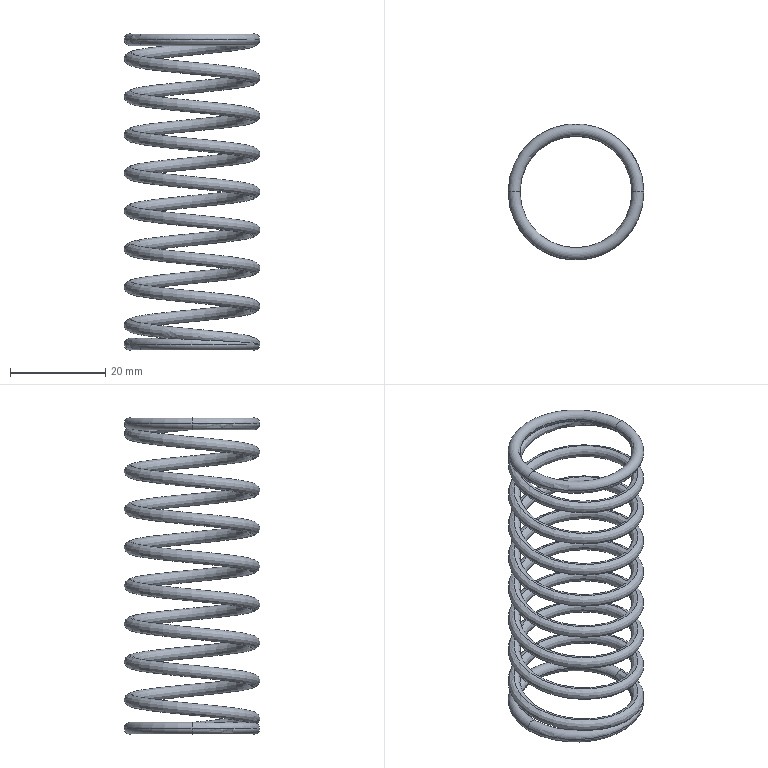Part | NX | features BREP 1 | 1 solid | 10 faces | box 28.5 x 28.5 x 66.5 mm | volume 3897 mm3 | torus 8 | spline 2